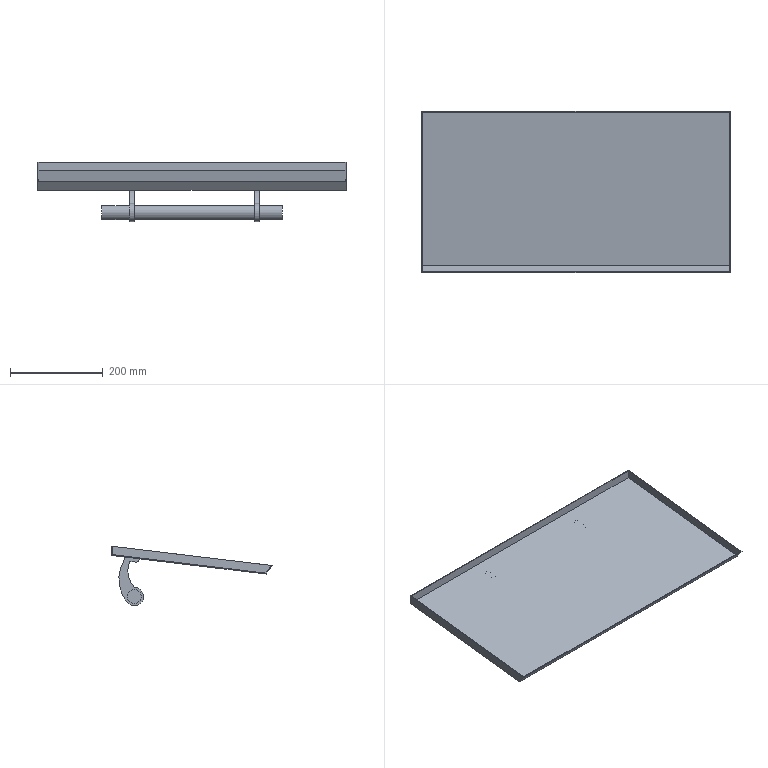Part | SolidWorks | features ICE 5, Extrusion 1, LPattern 1 | 1 solid | 35 faces | box 665 x 347.491 x 128.669 mm | volume 843762 mm3 | plane 21 | cylinder 10 | spline 4 | commonest cylinder face diameters 30 x6 14 x2 40 x2
STEP:
#1=CARTESIAN_POINT('',(-135.5,-49.466,-103.669));
#2=VERTEX_POINT('',#1);
#3=CARTESIAN_POINT('',(-135.5,-49.466,-73.669));
#4=VERTEX_POINT('',#3);
#5=CARTESIAN_POINT('',(-135.5,-49.466,-88.669));
#6=DIRECTION('',(1.,0.,0.));
#7=DIRECTION('',(0.,0.,-1.));
#8=AXIS2_PLACEMENT_3D('',#5,#6,#7);
#9=CIRCLE('',#8,15.);
#10=EDGE_CURVE('',#2,#4,#9,.T.);
#11=ORIENTED_EDGE('',*,*,#10,.F.);
#12=CARTESIAN_POINT('',(-185.5,-49.466,-103.669));
#13=VERTEX_POINT('',#12);
#14=CARTESIAN_POINT('',(-135.5,-49.466,-103.669));
#15=DIRECTION('',(-1.,0.,0.));
#16=VECTOR('',#15,1000.);
#17=LINE('',#14,#16);
#18=EDGE_CURVE('',#2,#13,#17,.T.);
#19=ORIENTED_EDGE('',*,*,#18,.T.);
#20=CARTESIAN_POINT('',(-185.5,-49.466,-73.669));
#21=VERTEX_POINT('',#20);
#22=CARTESIAN_POINT('',(-185.5,-49.466,-88.669));
#23=DIRECTION('',(1.,0.,0.));
#24=DIRECTION('',(0.,0.,-1.));
#25=AXIS2_PLACEMENT_3D('',#22,#23,#24);
#26=CIRCLE('',#25,15.);
#27=EDGE_CURVE('',#13,#21,#26,.T.);
#28=ORIENTED_EDGE('',*,*,#27,.T.);
#29=CARTESIAN_POINT('',(-135.5,-49.466,-73.669));
#30=DIRECTION('',(-1.,0.,0.));
#31=VECTOR('',#30,1000.);
#32=LINE('',#29,#31);
#33=EDGE_CURVE('',#4,#21,#32,.T.);
#34=ORIENTED_EDGE('',*,*,#33,.F.);
#35=EDGE_LOOP('',(#11,#19,#28,#34));
#36=FACE_OUTER_BOUND('',#35,.T.);
#37=CARTESIAN_POINT('',(-135.5,-49.466,-88.669));
#38=DIRECTION('',(-1.,0.,0.));
#39=DIRECTION('',(0.,0.,1.));
#40=AXIS2_PLACEMENT_3D('',#37,#38,#39);
#41=CYLINDRICAL_SURFACE('',#40,15.);
#42=ADVANCED_FACE('',(#36),#41,.T.);
#43=CARTESIAN_POINT('',(-455.5,-49.466,-103.669));
#44=VERTEX_POINT('',#43);
#45=CARTESIAN_POINT('',(-455.5,-49.466,-73.669));
#46=VERTEX_POINT('',#45);
#47=CARTESIAN_POINT('',(-455.5,-49.466,-88.669));
#48=DIRECTION('',(1.,0.,0.));
#49=DIRECTION('',(0.,0.,-1.));
#50=AXIS2_PLACEMENT_3D('',#47,#48,#49);
#51=CIRCLE('',#50,15.);
#52=EDGE_CURVE('',#44,#46,#51,.T.);
#53=ORIENTED_EDGE('',*,*,#52,.T.);
#54=CARTESIAN_POINT('',(-195.5,-49.466,-73.669));
#55=VERTEX_POINT('',#54);
#56=CARTESIAN_POINT('',(-525.5,-49.466,-73.669));
#57=DIRECTION('',(1.,0.,0.));
#58=VECTOR('',#57,1000.);
#59=LINE('',#56,#58);
#60=EDGE_CURVE('',#46,#55,#59,.T.);
#61=ORIENTED_EDGE('',*,*,#60,.T.);
#62=CARTESIAN_POINT('',(-195.5,-49.466,-103.669));
#63=VERTEX_POINT('',#62);
#64=CARTESIAN_POINT('',(-195.5,-49.466,-88.669));
#65=DIRECTION('',(1.,0.,0.));
#66=DIRECTION('',(0.,0.,-1.));
#67=AXIS2_PLACEMENT_3D('',#64,#65,#66);
#68=CIRCLE('',#67,15.);
#69=EDGE_CURVE('',#63,#55,#68,.T.);
#70=ORIENTED_EDGE('',*,*,#69,.F.);
#71=CARTESIAN_POINT('',(-525.5,-49.466,-103.669));
#72=DIRECTION('',(1.,0.,0.));
#73=VECTOR('',#72,1000.);
#74=LINE('',#71,#73);
#75=EDGE_CURVE('',#44,#63,#74,.T.);
#76=ORIENTED_EDGE('',*,*,#75,.F.);
#77=EDGE_LOOP('',(#53,#61,#70,#76));
#78=FACE_OUTER_BOUND('',#77,.T.);
#79=CARTESIAN_POINT('',(-525.5,-49.466,-88.669));
#80=DIRECTION('',(1.,0.,0.));
#81=DIRECTION('',(0.,0.,-1.));
#82=AXIS2_PLACEMENT_3D('',#79,#80,#81);
#83=CYLINDRICAL_SURFACE('',#82,15.);
#84=ADVANCED_FACE('',(#78),#83,.T.);
#85=CARTESIAN_POINT('',(-525.5,-49.466,-103.669));
#86=VERTEX_POINT('',#85);
#87=CARTESIAN_POINT('',(-525.5,-49.466,-73.669));
#88=VERTEX_POINT('',#87);
#89=CARTESIAN_POINT('',(-525.5,-49.466,-88.669));
#90=DIRECTION('',(1.,0.,0.));
#91=DIRECTION('',(0.,0.,-1.));
#92=AXIS2_PLACEMENT_3D('',#89,#90,#91);
#93=CIRCLE('',#92,15.);
#94=EDGE_CURVE('',#86,#88,#93,.T.);
#95=ORIENTED_EDGE('',*,*,#94,.T.);
#96=CARTESIAN_POINT('',(-465.5,-49.466,-73.669));
#97=VERTEX_POINT('',#96);
#98=CARTESIAN_POINT('',(-525.5,-49.466,-73.669));
#99=DIRECTION('',(1.,0.,0.));
#100=VECTOR('',#99,1000.);
#101=LINE('',#98,#100);
#102=EDGE_CURVE('',#88,#97,#101,.T.);
#103=ORIENTED_EDGE('',*,*,#102,.T.);
#104=CARTESIAN_POINT('',(-465.5,-49.466,-103.669));
#105=VERTEX_POINT('',#104);
#106=CARTESIAN_POINT('',(-465.5,-49.466,-88.669));
#107=DIRECTION('',(1.,0.,0.));
#108=DIRECTION('',(0.,0.,-1.));
#109=AXIS2_PLACEMENT_3D('',#106,#107,#108);
#110=CIRCLE('',#109,15.);
#111=EDGE_CURVE('',#105,#97,#110,.T.);
#112=ORIENTED_EDGE('',*,*,#111,.F.);
#113=CARTESIAN_POINT('',(-525.5,-49.466,-103.669));
#114=DIRECTION('',(1.,0.,0.));
#115=VECTOR('',#114,1000.);
#116=LINE('',#113,#115);
#117=EDGE_CURVE('',#86,#105,#116,.T.);
#118=ORIENTED_EDGE('',*,*,#117,.F.);
#119=EDGE_LOOP('',(#95,#103,#112,#118));
#120=FACE_OUTER_BOUND('',#119,.T.);
#121=CARTESIAN_POINT('',(-525.5,-49.466,-88.669));
#122=DIRECTION('',(1.,0.,0.));
#123=DIRECTION('',(0.,0.,-1.));
#124=AXIS2_PLACEMENT_3D('',#121,#122,#123);
#125=CYLINDRICAL_SURFACE('',#124,15.);
#126=ADVANCED_FACE('',(#120),#125,.T.);
#127=CARTESIAN_POINT('',(0.,-2.,1.774));
#128=VERTEX_POINT('',#127);
#129=CARTESIAN_POINT('',(0.,-2.,19.759));
#130=VERTEX_POINT('',#129);
#131=CARTESIAN_POINT('',(0.,-2.,1.774));
#132=DIRECTION('',(0.,0.,1.));
#133=VECTOR('',#132,1000.);
#134=LINE('',#131,#133);
#135=EDGE_CURVE('',#128,#130,#134,.T.);
#136=ORIENTED_EDGE('',*,*,#135,.F.);
#137=CARTESIAN_POINT('',(0.,-332.828,-38.054));
#138=VERTEX_POINT('',#137);
#139=CARTESIAN_POINT('',(0.,-332.828,-38.054));
#140=DIRECTION('',(0.,0.9928,0.1195));
#141=VECTOR('',#140,1000.);
#142=LINE('',#139,#141);
#143=EDGE_CURVE('',#138,#128,#142,.T.);
#144=ORIENTED_EDGE('',*,*,#143,.F.);
#145=CARTESIAN_POINT('',(0.,-345.198,-21.558));
#146=VERTEX_POINT('',#145);
#147=CARTESIAN_POINT('',(0.,-345.198,-21.558));
#148=DIRECTION('',(0.,0.5999,-0.8001));
#149=VECTOR('',#148,1000.);
#150=LINE('',#147,#149);
#151=EDGE_CURVE('',#146,#138,#150,.T.);
#152=ORIENTED_EDGE('',*,*,#151,.F.);
#153=CARTESIAN_POINT('',(0.,0.,20.));
#154=DIRECTION('',(0.,-0.9928,-0.1195));
#155=VECTOR('',#154,1000.);
#156=LINE('',#153,#155);
#157=EDGE_CURVE('',#130,#146,#156,.T.);
#158=ORIENTED_EDGE('',*,*,#157,.F.);
#159=EDGE_LOOP('',(#136,#144,#152,#158));
#160=FACE_OUTER_BOUND('',#159,.T.);
#161=CARTESIAN_POINT('',(0.,0.,0.));
#162=DIRECTION('',(1.,0.,0.));
#163=DIRECTION('',(0.,0.,-1.));
#164=AXIS2_PLACEMENT_3D('',#161,#162,#163);
#165=PLANE('',#164);
#166=ADVANCED_FACE('',(#160),#165,.F.);
#167=CARTESIAN_POINT('',(-455.5,-60.424,-7.274));
#168=VERTEX_POINT('',#167);
#169=CARTESIAN_POINT('',(-465.5,-60.424,-7.274));
#170=VERTEX_POINT('',#169);
#171=CARTESIAN_POINT('',(-455.5,-60.424,-7.274));
#172=DIRECTION('',(-1.,0.,0.));
#173=VECTOR('',#172,1000.);
#174=LINE('',#171,#173);
#175=EDGE_CURVE('',#168,#170,#174,.T.);
#176=ORIENTED_EDGE('',*,*,#175,.F.);
#177=CARTESIAN_POINT('',(-455.5,-29.965,-3.607));
#178=VERTEX_POINT('',#177);
#179=CARTESIAN_POINT('',(-455.5,0.,0.));
#180=DIRECTION('',(0.,0.9928,0.1195));
#181=VECTOR('',#180,1000.);
#182=LINE('',#179,#181);
#183=EDGE_CURVE('',#168,#178,#182,.T.);
#184=ORIENTED_EDGE('',*,*,#183,.T.);
#185=CARTESIAN_POINT('',(-465.5,-29.965,-3.607));
#186=VERTEX_POINT('',#185);
#187=CARTESIAN_POINT('',(-455.5,-29.965,-3.607));
#188=DIRECTION('',(-1.,0.,0.));
#189=VECTOR('',#188,1000.);
#190=LINE('',#187,#189);
#191=EDGE_CURVE('',#178,#186,#190,.T.);
#192=ORIENTED_EDGE('',*,*,#191,.T.);
#193=CARTESIAN_POINT('',(-465.5,0.,0.));
#194=DIRECTION('',(0.,0.9928,0.1195));
#195=VECTOR('',#194,1000.);
#196=LINE('',#193,#195);
#197=EDGE_CURVE('',#170,#186,#196,.T.);
#198=ORIENTED_EDGE('',*,*,#197,.F.);
#199=EDGE_LOOP('',(#176,#184,#192,#198));
#200=FACE_BOUND('',#199,.T.);
#201=CARTESIAN_POINT('',(-185.5,-60.424,-7.274));
#202=VERTEX_POINT('',#201);
#203=CARTESIAN_POINT('',(-195.5,-60.424,-7.274));
#204=VERTEX_POINT('',#203);
#205=CARTESIAN_POINT('',(-185.5,-60.424,-7.274));
#206=DIRECTION('',(-1.,0.,0.));
#207=VECTOR('',#206,1000.);
#208=LINE('',#205,#207);
#209=EDGE_CURVE('',#202,#204,#208,.T.);
#210=ORIENTED_EDGE('',*,*,#209,.F.);
#211=CARTESIAN_POINT('',(-185.5,-29.965,-3.607));
#212=VERTEX_POINT('',#211);
#213=CARTESIAN_POINT('',(-185.5,0.,0.));
#214=DIRECTION('',(0.,0.9928,0.1195));
#215=VECTOR('',#214,1000.);
#216=LINE('',#213,#215);
#217=EDGE_CURVE('',#202,#212,#216,.T.);
#218=ORIENTED_EDGE('',*,*,#217,.T.);
#219=CARTESIAN_POINT('',(-195.5,-29.965,-3.607));
#220=VERTEX_POINT('',#219);
#221=CARTESIAN_POINT('',(-185.5,-29.965,-3.607));
#222=DIRECTION('',(-1.,0.,0.));
#223=VECTOR('',#222,1000.);
#224=LINE('',#221,#223);
#225=EDGE_CURVE('',#212,#220,#224,.T.);
#226=ORIENTED_EDGE('',*,*,#225,.T.);
#227=CARTESIAN_POINT('',(-195.5,0.,0.));
#228=DIRECTION('',(0.,0.9928,0.1195));
#229=VECTOR('',#228,1000.);
#230=LINE('',#227,#229);
#231=EDGE_CURVE('',#204,#220,#230,.T.);
#232=ORIENTED_EDGE('',*,*,#231,.F.);
#233=EDGE_LOOP('',(#210,#218,#226,#232));
#234=FACE_BOUND('',#233,.T.);
#235=CARTESIAN_POINT('',(2.,-333.735,-40.178));
#236=VERTEX_POINT('',#235);
#237=CARTESIAN_POINT('',(-663.,-333.735,-40.178));
#238=VERTEX_POINT('',#237);
#239=CARTESIAN_POINT('',(2.,-333.735,-40.178));
#240=DIRECTION('',(-1.,0.,0.));
#241=VECTOR('',#240,1000.);
#242=LINE('',#239,#241);
#243=EDGE_CURVE('',#236,#238,#242,.T.);
#244=ORIENTED_EDGE('',*,*,#243,.T.);
#245=CARTESIAN_POINT('',(-663.,0.,0.));
#246=VERTEX_POINT('',#245);
#247=CARTESIAN_POINT('',(-663.,0.,0.));
#248=DIRECTION('',(0.,-0.9928,-0.1195));
#249=VECTOR('',#248,1000.);
#250=LINE('',#247,#249);
#251=EDGE_CURVE('',#246,#238,#250,.T.);
#252=ORIENTED_EDGE('',*,*,#251,.F.);
#253=CARTESIAN_POINT('',(2.,0.,0.));
#254=VERTEX_POINT('',#253);
#255=CARTESIAN_POINT('',(2.,0.,0.));
#256=DIRECTION('',(-1.,0.,0.));
#257=VECTOR('',#256,1000.);
#258=LINE('',#255,#257);
#259=EDGE_CURVE('',#254,#246,#258,.T.);
#260=ORIENTED_EDGE('',*,*,#259,.F.);
#261=CARTESIAN_POINT('',(2.,-333.735,-40.178));
#262=DIRECTION('',(0.,0.9928,0.1195));
#263=VECTOR('',#262,1000.);
#264=LINE('',#261,#263);
#265=EDGE_CURVE('',#236,#254,#264,.T.);
#266=ORIENTED_EDGE('',*,*,#265,.F.);
#267=EDGE_LOOP('',(#244,#252,#260,#266));
#268=FACE_OUTER_BOUND('',#267,.T.);
#269=CARTESIAN_POINT('',(2.,-333.735,-40.178));
#270=DIRECTION('',(0.,-0.1195,0.9928));
#271=DIRECTION('',(0.,-0.9928,-0.1195));
#272=AXIS2_PLACEMENT_3D('',#269,#270,#271);
#273=PLANE('',#272);
#274=ADVANCED_FACE('',(#200,#234,#268),#273,.F.);
#275=ORIENTED_EDGE('',*,*,#259,.T.);
#276=CARTESIAN_POINT('',(-663.,0.,20.));
#277=VERTEX_POINT('',#276);
#278=CARTESIAN_POINT('',(-663.,0.,20.));
#279=DIRECTION('',(0.,0.,-1.));
#280=VECTOR('',#279,1000.);
#281=LINE('',#278,#280);
#282=EDGE_CURVE('',#277,#246,#281,.T.);
#283=ORIENTED_EDGE('',*,*,#282,.F.);
#284=CARTESIAN_POINT('',(2.,0.,20.));
#285=VERTEX_POINT('',#284);
#286=CARTESIAN_POINT('',(2.,0.,20.));
#287=DIRECTION('',(-1.,0.,0.));
#288=VECTOR('',#287,1000.);
#289=LINE('',#286,#288);
#290=EDGE_CURVE('',#285,#277,#289,.T.);
#291=ORIENTED_EDGE('',*,*,#290,.F.);
#292=CARTESIAN_POINT('',(2.,0.,0.));
#293=DIRECTION('',(0.,0.,1.));
#294=VECTOR('',#293,1000.);
#295=LINE('',#292,#294);
#296=EDGE_CURVE('',#254,#285,#295,.T.);
#297=ORIENTED_EDGE('',*,*,#296,.F.);
#298=EDGE_LOOP('',(#275,#283,#291,#297));
#299=FACE_OUTER_BOUND('',#298,.T.);
#300=CARTESIAN_POINT('',(2.,0.,0.));
#301=DIRECTION('',(0.,-1.,0.));
#302=DIRECTION('',(0.,0.,-1.));
#303=AXIS2_PLACEMENT_3D('',#300,#301,#302);
#304=PLANE('',#303);
#305=ADVANCED_FACE('',(#299),#304,.F.);
#306=CARTESIAN_POINT('',(-661.,-345.198,-21.558));
#307=VERTEX_POINT('',#306);
#308=CARTESIAN_POINT('',(-661.,-345.198,-21.558));
#309=DIRECTION('',(1.,0.,0.));
#310=VECTOR('',#309,1000.);
#311=LINE('',#308,#310);
#312=EDGE_CURVE('',#307,#146,#311,.T.);
#313=ORIENTED_EDGE('',*,*,#312,.F.);
#314=CARTESIAN_POINT('',(-661.,-2.,19.759));
#315=VERTEX_POINT('',#314);
#316=CARTESIAN_POINT('',(-661.,-347.491,-21.834));
#317=DIRECTION('',(0.,0.9928,0.1195));
#318=VECTOR('',#317,1000.);
#319=LINE('',#316,#318);
#320=EDGE_CURVE('',#307,#315,#319,.T.);
#321=ORIENTED_EDGE('',*,*,#320,.T.);
#322=CARTESIAN_POINT('',(-661.,-2.,19.759));
#323=DIRECTION('',(1.,0.,0.));
#324=VECTOR('',#323,1000.);
#325=LINE('',#322,#324);
#326=EDGE_CURVE('',#315,#130,#325,.T.);
#327=ORIENTED_EDGE('',*,*,#326,.T.);
#328=ORIENTED_EDGE('',*,*,#157,.T.);
#329=EDGE_LOOP('',(#313,#321,#327,#328));
#330=FACE_BOUND('',#329,.T.);
#331=ORIENTED_EDGE('',*,*,#290,.T.);
#332=CARTESIAN_POINT('',(-663.,-347.491,-21.834));
#333=VERTEX_POINT('',#332);
#334=CARTESIAN_POINT('',(-663.,-347.491,-21.834));
#335=DIRECTION('',(0.,0.9928,0.1195));
#336=VECTOR('',#335,1000.);
#337=LINE('',#334,#336);
#338=EDGE_CURVE('',#333,#277,#337,.T.);
#339=ORIENTED_EDGE('',*,*,#338,.F.);
#340=CARTESIAN_POINT('',(2.,-347.491,-21.834));
#341=VERTEX_POINT('',#340);
#342=CARTESIAN_POINT('',(2.,-347.491,-21.834));
#343=DIRECTION('',(-1.,0.,0.));
#344=VECTOR('',#343,1000.);
#345=LINE('',#342,#344);
#346=EDGE_CURVE('',#341,#333,#345,.T.);
#347=ORIENTED_EDGE('',*,*,#346,.F.);
#348=CARTESIAN_POINT('',(2.,0.,20.));
#349=DIRECTION('',(0.,-0.9928,-0.1195));
#350=VECTOR('',#349,1000.);
#351=LINE('',#348,#350);
#352=EDGE_CURVE('',#285,#341,#351,.T.);
#353=ORIENTED_EDGE('',*,*,#352,.F.);
#354=EDGE_LOOP('',(#331,#339,#347,#353));
#355=FACE_OUTER_BOUND('',#354,.T.);
#356=CARTESIAN_POINT('',(2.,0.,20.));
#357=DIRECTION('',(0.,0.1195,-0.9928));
#358=DIRECTION('',(0.,0.9928,0.1195));
#359=AXIS2_PLACEMENT_3D('',#356,#357,#358);
#360=PLANE('',#359);
#361=ADVANCED_FACE('',(#330,#355),#360,.F.);
#362=ORIENTED_EDGE('',*,*,#346,.T.);
#363=CARTESIAN_POINT('',(-663.,-333.735,-40.178));
#364=DIRECTION('',(0.,-0.5999,0.8001));
#365=VECTOR('',#364,1000.);
#366=LINE('',#363,#365);
#367=EDGE_CURVE('',#238,#333,#366,.T.);
#368=ORIENTED_EDGE('',*,*,#367,.F.);
#369=ORIENTED_EDGE('',*,*,#243,.F.);
#370=CARTESIAN_POINT('',(2.,-347.491,-21.834));
#371=DIRECTION('',(0.,0.5999,-0.8001));
#372=VECTOR('',#371,1000.);
#373=LINE('',#370,#372);
#374=EDGE_CURVE('',#341,#236,#373,.T.);
#375=ORIENTED_EDGE('',*,*,#374,.F.);
#376=EDGE_LOOP('',(#362,#368,#369,#375));
#377=FACE_OUTER_BOUND('',#376,.T.);
#378=CARTESIAN_POINT('',(2.,-347.491,-21.834));
#379=DIRECTION('',(0.,0.8001,0.5999));
#380=DIRECTION('',(0.,-0.5999,0.8001));
#381=AXIS2_PLACEMENT_3D('',#378,#379,#380);
#382=PLANE('',#381);
#383=ADVANCED_FACE('',(#377),#382,.F.);
#384=ORIENTED_EDGE('',*,*,#265,.T.);
#385=ORIENTED_EDGE('',*,*,#296,.T.);
#386=ORIENTED_EDGE('',*,*,#352,.T.);
#387=ORIENTED_EDGE('',*,*,#374,.T.);
#388=EDGE_LOOP('',(#384,#385,#386,#387));
#389=FACE_OUTER_BOUND('',#388,.T.);
#390=CARTESIAN_POINT('',(2.,0.,0.));
#391=DIRECTION('',(1.,0.,0.));
#392=DIRECTION('',(0.,0.,-1.));
#393=AXIS2_PLACEMENT_3D('',#390,#391,#392);
#394=PLANE('',#393);
#395=ADVANCED_FACE('',(#389),#394,.T.);
#396=ORIENTED_EDGE('',*,*,#151,.T.);
#397=CARTESIAN_POINT('',(-661.,-332.828,-38.054));
#398=VERTEX_POINT('',#397);
#399=CARTESIAN_POINT('',(-661.,-332.828,-38.054));
#400=DIRECTION('',(1.,0.,0.));
#401=VECTOR('',#400,1000.);
#402=LINE('',#399,#401);
#403=EDGE_CURVE('',#398,#138,#402,.T.);
#404=ORIENTED_EDGE('',*,*,#403,.F.);
#405=CARTESIAN_POINT('',(-661.,-345.198,-21.558));
#406=DIRECTION('',(0.,0.5999,-0.8001));
#407=VECTOR('',#406,1000.);
#408=LINE('',#405,#407);
#409=EDGE_CURVE('',#307,#398,#408,.T.);
#410=ORIENTED_EDGE('',*,*,#409,.F.);
#411=ORIENTED_EDGE('',*,*,#312,.T.);
#412=EDGE_LOOP('',(#396,#404,#410,#411));
#413=FACE_OUTER_BOUND('',#412,.T.);
#414=CARTESIAN_POINT('',(-661.,-345.198,-21.558));
#415=DIRECTION('',(0.,-0.8001,-0.5999));
#416=DIRECTION('',(0.,0.5999,-0.8001));
#417=AXIS2_PLACEMENT_3D('',#414,#415,#416);
#418=PLANE('',#417);
#419=ADVANCED_FACE('',(#413),#418,.F.);
#420=ORIENTED_EDGE('',*,*,#143,.T.);
#421=CARTESIAN_POINT('',(-661.,-2.,1.774));
#422=VERTEX_POINT('',#421);
#423=CARTESIAN_POINT('',(-661.,-2.,1.774));
#424=DIRECTION('',(1.,0.,0.));
#425=VECTOR('',#424,1000.);
#426=LINE('',#423,#425);
#427=EDGE_CURVE('',#422,#128,#426,.T.);
#428=ORIENTED_EDGE('',*,*,#427,.F.);
#429=CARTESIAN_POINT('',(-661.,-332.828,-38.054));
#430=DIRECTION('',(0.,0.9928,0.1195));
#431=VECTOR('',#430,1000.);
#432=LINE('',#429,#431);
#433=EDGE_CURVE('',#398,#422,#432,.T.);
#434=ORIENTED_EDGE('',*,*,#433,.F.);
#435=ORIENTED_EDGE('',*,*,#403,.T.);
#436=EDGE_LOOP('',(#420,#428,#434,#435));
#437=FACE_OUTER_BOUND('',#436,.T.);
#438=CARTESIAN_POINT('',(-661.,-332.828,-38.054));
#439=DIRECTION('',(0.,0.1195,-0.9928));
#440=DIRECTION('',(0.,0.9928,0.1195));
#441=AXIS2_PLACEMENT_3D('',#438,#439,#440);
#442=PLANE('',#441);
#443=ADVANCED_FACE('',(#437),#442,.F.);
#444=ORIENTED_EDGE('',*,*,#135,.T.);
#445=ORIENTED_EDGE('',*,*,#326,.F.);
#446=CARTESIAN_POINT('',(-661.,-2.,1.774));
#447=DIRECTION('',(0.,0.,1.));
#448=VECTOR('',#447,1000.);
#449=LINE('',#446,#448);
#450=EDGE_CURVE('',#422,#315,#449,.T.);
#451=ORIENTED_EDGE('',*,*,#450,.F.);
#452=ORIENTED_EDGE('',*,*,#427,.T.);
#453=EDGE_LOOP('',(#444,#445,#451,#452));
#454=FACE_OUTER_BOUND('',#453,.T.);
#455=CARTESIAN_POINT('',(-661.,-2.,1.774));
#456=DIRECTION('',(0.,1.,0.));
#457=DIRECTION('',(0.,0.,1.));
#458=AXIS2_PLACEMENT_3D('',#455,#456,#457);
#459=PLANE('',#458);
#460=ADVANCED_FACE('',(#454),#459,.F.);
#461=ORIENTED_EDGE('',*,*,#251,.T.);
#462=ORIENTED_EDGE('',*,*,#367,.T.);
#463=ORIENTED_EDGE('',*,*,#338,.T.);
#464=ORIENTED_EDGE('',*,*,#282,.T.);
#465=EDGE_LOOP('',(#461,#462,#463,#464));
#466=FACE_OUTER_BOUND('',#465,.T.);
#467=CARTESIAN_POINT('',(-663.,0.,0.));
#468=DIRECTION('',(1.,0.,0.));
#469=DIRECTION('',(0.,0.,-1.));
#470=AXIS2_PLACEMENT_3D('',#467,#468,#469);
#471=PLANE('',#470);
#472=ADVANCED_FACE('',(#466),#471,.F.);
#473=ORIENTED_EDGE('',*,*,#320,.F.);
#474=ORIENTED_EDGE('',*,*,#409,.T.);
#475=ORIENTED_EDGE('',*,*,#433,.T.);
#476=ORIENTED_EDGE('',*,*,#450,.T.);
#477=EDGE_LOOP('',(#473,#474,#475,#476));
#478=FACE_OUTER_BOUND('',#477,.T.);
#479=CARTESIAN_POINT('',(-661.,0.,0.));
#480=DIRECTION('',(1.,0.,0.));
#481=DIRECTION('',(0.,0.,-1.));
#482=AXIS2_PLACEMENT_3D('',#479,#480,#481);
#483=PLANE('',#482);
#484=ADVANCED_FACE('',(#478),#483,.T.);
#485=CARTESIAN_POINT('',(-195.5,-49.466,-68.669));
#486=VERTEX_POINT('',#485);
#487=CARTESIAN_POINT('',(-195.5,-33.713,-100.991));
#488=VERTEX_POINT('',#487);
#489=CARTESIAN_POINT('',(-195.5,-49.466,-88.669));
#490=DIRECTION('',(1.,0.,0.));
#491=DIRECTION('',(0.,0.,-1.));
#492=AXIS2_PLACEMENT_3D('',#489,#490,#491);
#493=CIRCLE('',#492,20.);
#494=EDGE_CURVE('',#486,#488,#493,.T.);
#495=ORIENTED_EDGE('',*,*,#494,.T.);
#496=CARTESIAN_POINT('',(-185.5,-33.713,-100.991));
#497=VERTEX_POINT('',#496);
#498=CARTESIAN_POINT('',(-185.5,-33.713,-100.991));
#499=DIRECTION('',(-1.,0.,0.));
#500=VECTOR('',#499,1000.);
#501=LINE('',#498,#500);
#502=EDGE_CURVE('',#497,#488,#501,.T.);
#503=ORIENTED_EDGE('',*,*,#502,.F.);
#504=CARTESIAN_POINT('',(-185.5,-49.466,-68.669));
#505=VERTEX_POINT('',#504);
#506=CARTESIAN_POINT('',(-185.5,-49.466,-88.669));
#507=DIRECTION('',(1.,0.,0.));
#508=DIRECTION('',(0.,0.,-1.));
#509=AXIS2_PLACEMENT_3D('',#506,#507,#508);
#510=CIRCLE('',#509,20.);
#511=EDGE_CURVE('',#505,#497,#510,.T.);
#512=ORIENTED_EDGE('',*,*,#511,.F.);
#513=CARTESIAN_POINT('',(-185.5,-49.466,-68.669));
#514=DIRECTION('',(-1.,0.,0.));
#515=VECTOR('',#514,1000.);
#516=LINE('',#513,#515);
#517=EDGE_CURVE('',#505,#486,#516,.T.);
#518=ORIENTED_EDGE('',*,*,#517,.T.);
#519=EDGE_LOOP('',(#495,#503,#512,#518));
#520=FACE_OUTER_BOUND('',#519,.T.);
#521=CARTESIAN_POINT('',(-185.5,-49.466,-88.669));
#522=DIRECTION('',(-1.,0.,0.));
#523=DIRECTION('',(0.,0.,1.));
#524=AXIS2_PLACEMENT_3D('',#521,#522,#523);
#525=CYLINDRICAL_SURFACE('',#524,20.);
#526=ADVANCED_FACE('',(#520),#525,.T.);
#527=CARTESIAN_POINT('',(-195.5,-29.965,-3.607));
#528=CARTESIAN_POINT('',(-195.5,-12.413,-33.423));
#529=CARTESIAN_POINT('',(-195.5,-8.887,-69.251));
#530=CARTESIAN_POINT('',(-195.5,-33.713,-100.991));
#531=B_SPLINE_CURVE_WITH_KNOTS('',3,(#527,#528,#529,#530),.UNSPECIFIED.,.F.,.F.,(4,4),(0.,1.),.UNSPECIFIED.);
#532=EDGE_CURVE('',#220,#488,#531,.T.);
#533=ORIENTED_EDGE('',*,*,#532,.F.);
#534=ORIENTED_EDGE('',*,*,#225,.F.);
#535=CARTESIAN_POINT('',(-185.5,-29.965,-3.607));
#536=CARTESIAN_POINT('',(-185.5,-12.413,-33.423));
#537=CARTESIAN_POINT('',(-185.5,-8.887,-69.251));
#538=CARTESIAN_POINT('',(-185.5,-33.713,-100.991));
#539=B_SPLINE_CURVE_WITH_KNOTS('',3,(#535,#536,#537,#538),.UNSPECIFIED.,.F.,.F.,(4,4),(0.,1.),.UNSPECIFIED.);
#540=EDGE_CURVE('',#212,#497,#539,.T.);
#541=ORIENTED_EDGE('',*,*,#540,.T.);
#542=ORIENTED_EDGE('',*,*,#502,.T.);
#543=EDGE_LOOP('',(#533,#534,#541,#542));
#544=FACE_OUTER_BOUND('',#543,.T.);
#545=CARTESIAN_POINT('',(-185.5,-29.965,-3.607));
#546=CARTESIAN_POINT('',(-195.5,-29.965,-3.607));
#547=CARTESIAN_POINT('',(-185.5,-12.413,-33.423));
#548=CARTESIAN_POINT('',(-195.5,-12.413,-33.423));
#549=CARTESIAN_POINT('',(-185.5,-8.887,-69.251));
#550=CARTESIAN_POINT('',(-195.5,-8.887,-69.251));
#551=CARTESIAN_POINT('',(-185.5,-33.713,-100.991));
#552=CARTESIAN_POINT('',(-195.5,-33.713,-100.991));
#553=B_SPLINE_SURFACE_WITH_KNOTS('',3,1,((#545,#546),(#547,#548),(#549,#550),(#551,#552)),.UNSPECIFIED.,.F.,.F.,.F.,(4,4),(2,2),(0.,1.),(0.,1.),.UNSPECIFIED.);
#554=ADVANCED_FACE('',(#544),#553,.T.);
#555=CARTESIAN_POINT('',(-195.5,-60.305,-8.267));
#556=VERTEX_POINT('',#555);
#557=CARTESIAN_POINT('',(-195.5,-60.424,-7.274));
#558=DIRECTION('',(0.,0.1195,-0.9928));
#559=VECTOR('',#558,1000.);
#560=LINE('',#557,#559);
#561=EDGE_CURVE('',#204,#556,#560,.T.);
#562=ORIENTED_EDGE('',*,*,#561,.T.);
#563=CARTESIAN_POINT('',(-185.5,-60.305,-8.267));
#564=VERTEX_POINT('',#563);
#565=CARTESIAN_POINT('',(-185.5,-60.305,-8.267));
#566=DIRECTION('',(-1.,0.,0.));
#567=VECTOR('',#566,1000.);
#568=LINE('',#565,#567);
#569=EDGE_CURVE('',#564,#556,#568,.T.);
#570=ORIENTED_EDGE('',*,*,#569,.F.);
#571=CARTESIAN_POINT('',(-185.5,-60.424,-7.274));
#572=DIRECTION('',(0.,0.1195,-0.9928));
#573=VECTOR('',#572,1000.);
#574=LINE('',#571,#573);
#575=EDGE_CURVE('',#202,#564,#574,.T.);
#576=ORIENTED_EDGE('',*,*,#575,.F.);
#577=ORIENTED_EDGE('',*,*,#209,.T.);
#578=EDGE_LOOP('',(#562,#570,#576,#577));
#579=FACE_OUTER_BOUND('',#578,.T.);
#580=CARTESIAN_POINT('',(-185.5,-60.424,-7.274));
#581=DIRECTION('',(0.,0.9928,0.1195));
#582=DIRECTION('',(0.,-0.1195,0.9928));
#583=AXIS2_PLACEMENT_3D('',#580,#581,#582);
#584=PLANE('',#583);
#585=ADVANCED_FACE('',(#579),#584,.F.);
#586=CARTESIAN_POINT('',(-195.5,-52.518,-14.38));
#587=VERTEX_POINT('',#586);
#588=CARTESIAN_POINT('',(-195.5,-53.355,-7.431));
#589=DIRECTION('',(-1.,0.,0.));
#590=DIRECTION('',(0.,0.,-1.));
#591=AXIS2_PLACEMENT_3D('',#588,#589,#590);
#592=CIRCLE('',#591,7.);
#593=EDGE_CURVE('',#587,#556,#592,.T.);
#594=ORIENTED_EDGE('',*,*,#593,.F.);
#595=CARTESIAN_POINT('',(-185.5,-52.518,-14.38));
#596=VERTEX_POINT('',#595);
#597=CARTESIAN_POINT('',(-185.5,-52.518,-14.38));
#598=DIRECTION('',(-1.,0.,0.));
#599=VECTOR('',#598,1000.);
#600=LINE('',#597,#599);
#601=EDGE_CURVE('',#596,#587,#600,.T.);
#602=ORIENTED_EDGE('',*,*,#601,.F.);
#603=CARTESIAN_POINT('',(-185.5,-53.355,-7.431));
#604=DIRECTION('',(-1.,0.,0.));
#605=DIRECTION('',(0.,0.,-1.));
#606=AXIS2_PLACEMENT_3D('',#603,#604,#605);
#607=CIRCLE('',#606,7.);
#608=EDGE_CURVE('',#596,#564,#607,.T.);
#609=ORIENTED_EDGE('',*,*,#608,.T.);
#610=ORIENTED_EDGE('',*,*,#569,.T.);
#611=EDGE_LOOP('',(#594,#602,#609,#610));
#612=FACE_OUTER_BOUND('',#611,.T.);
#613=CARTESIAN_POINT('',(-185.5,-53.355,-7.431));
#614=DIRECTION('',(-1.,0.,0.));
#615=DIRECTION('',(0.,0.,1.));
#616=AXIS2_PLACEMENT_3D('',#613,#614,#615);
#617=CYLINDRICAL_SURFACE('',#616,7.);
#618=ADVANCED_FACE('',(#612),#617,.T.);
#619=CARTESIAN_POINT('',(-195.5,-39.608,-12.826));
#620=VERTEX_POINT('',#619);
#621=CARTESIAN_POINT('',(-195.5,0.9562,-7.943));
#622=DIRECTION('',(0.,0.9928,0.1195));
#623=VECTOR('',#622,1000.);
#624=LINE('',#621,#623);
#625=EDGE_CURVE('',#587,#620,#624,.T.);
#626=ORIENTED_EDGE('',*,*,#625,.T.);
#627=CARTESIAN_POINT('',(-185.5,-39.608,-12.826));
#628=VERTEX_POINT('',#627);
#629=CARTESIAN_POINT('',(-185.5,-39.608,-12.826));
#630=DIRECTION('',(-1.,0.,0.));
#631=VECTOR('',#630,1000.);
#632=LINE('',#629,#631);
#633=EDGE_CURVE('',#628,#620,#632,.T.);
#634=ORIENTED_EDGE('',*,*,#633,.F.);
#635=CARTESIAN_POINT('',(-185.5,0.9562,-7.943));
#636=DIRECTION('',(0.,0.9928,0.1195));
#637=VECTOR('',#636,1000.);
#638=LINE('',#635,#637);
#639=EDGE_CURVE('',#596,#628,#638,.T.);
#640=ORIENTED_EDGE('',*,*,#639,.F.);
#641=ORIENTED_EDGE('',*,*,#601,.T.);
#642=EDGE_LOOP('',(#626,#634,#640,#641));
#643=FACE_OUTER_BOUND('',#642,.T.);
#644=CARTESIAN_POINT('',(-185.5,0.9562,-7.943));
#645=DIRECTION('',(0.,-0.1195,0.9928));
#646=DIRECTION('',(0.,-0.9928,-0.1195));
#647=AXIS2_PLACEMENT_3D('',#644,#645,#646);
#648=PLANE('',#647);
#649=ADVANCED_FACE('',(#643),#648,.F.);
#650=CARTESIAN_POINT('',(-195.5,-39.608,-12.826));
#651=CARTESIAN_POINT('',(-195.5,-27.323,-40.794));
#652=CARTESIAN_POINT('',(-195.5,-49.466,-68.669));
#653=B_SPLINE_CURVE_WITH_KNOTS('',2,(#650,#651,#652),.UNSPECIFIED.,.F.,.F.,(3,3),(0.,1.),.UNSPECIFIED.);
#654=EDGE_CURVE('',#620,#486,#653,.T.);
#655=ORIENTED_EDGE('',*,*,#654,.T.);
#656=ORIENTED_EDGE('',*,*,#517,.F.);
#657=CARTESIAN_POINT('',(-185.5,-39.608,-12.826));
#658=CARTESIAN_POINT('',(-185.5,-27.323,-40.794));
#659=CARTESIAN_POINT('',(-185.5,-49.466,-68.669));
#660=B_SPLINE_CURVE_WITH_KNOTS('',2,(#657,#658,#659),.UNSPECIFIED.,.F.,.F.,(3,3),(0.,1.),.UNSPECIFIED.);
#661=EDGE_CURVE('',#628,#505,#660,.T.);
#662=ORIENTED_EDGE('',*,*,#661,.F.);
#663=ORIENTED_EDGE('',*,*,#633,.T.);
#664=EDGE_LOOP('',(#655,#656,#662,#663));
#665=FACE_OUTER_BOUND('',#664,.T.);
#666=CARTESIAN_POINT('',(-185.5,-39.608,-12.826));
#667=CARTESIAN_POINT('',(-195.5,-39.608,-12.826));
#668=CARTESIAN_POINT('',(-185.5,-27.323,-40.794));
#669=CARTESIAN_POINT('',(-195.5,-27.323,-40.794));
#670=CARTESIAN_POINT('',(-185.5,-49.466,-68.669));
#671=CARTESIAN_POINT('',(-195.5,-49.466,-68.669));
#672=B_SPLINE_SURFACE_WITH_KNOTS('',2,1,((#666,#667),(#668,#669),(#670,#671)),.UNSPECIFIED.,.F.,.F.,.F.,(3,3),(2,2),(0.,1.),(0.,1.),.UNSPECIFIED.);
#673=ADVANCED_FACE('',(#665),#672,.F.);
#674=CARTESIAN_POINT('',(-185.5,-49.466,-88.669));
#675=DIRECTION('',(1.,0.,0.));
#676=DIRECTION('',(0.,0.,-1.));
#677=AXIS2_PLACEMENT_3D('',#674,#675,#676);
#678=CIRCLE('',#677,15.);
#679=EDGE_CURVE('',#21,#13,#678,.T.);
#680=ORIENTED_EDGE('',*,*,#679,.F.);
#681=ORIENTED_EDGE('',*,*,#27,.F.);
#682=EDGE_LOOP('',(#680,#681));
#683=FACE_BOUND('',#682,.T.);
#684=ORIENTED_EDGE('',*,*,#511,.T.);
#685=ORIENTED_EDGE('',*,*,#540,.F.);
#686=ORIENTED_EDGE('',*,*,#217,.F.);
#687=ORIENTED_EDGE('',*,*,#575,.T.);
#688=ORIENTED_EDGE('',*,*,#608,.F.);
#689=ORIENTED_EDGE('',*,*,#639,.T.);
#690=ORIENTED_EDGE('',*,*,#661,.T.);
#691=EDGE_LOOP('',(#684,#685,#686,#687,#688,#689,#690));
#692=FACE_OUTER_BOUND('',#691,.T.);
#693=CARTESIAN_POINT('',(-185.5,0.,0.));
#694=DIRECTION('',(1.,0.,0.));
#695=DIRECTION('',(0.,0.,-1.));
#696=AXIS2_PLACEMENT_3D('',#693,#694,#695);
#697=PLANE('',#696);
#698=ADVANCED_FACE('',(#683,#692),#697,.T.);
#699=ORIENTED_EDGE('',*,*,#69,.T.);
#700=CARTESIAN_POINT('',(-195.5,-49.466,-88.669));
#701=DIRECTION('',(1.,0.,0.));
#702=DIRECTION('',(0.,0.,-1.));
#703=AXIS2_PLACEMENT_3D('',#700,#701,#702);
#704=CIRCLE('',#703,15.);
#705=EDGE_CURVE('',#55,#63,#704,.T.);
#706=ORIENTED_EDGE('',*,*,#705,.T.);
#707=EDGE_LOOP('',(#699,#706));
#708=FACE_BOUND('',#707,.T.);
#709=ORIENTED_EDGE('',*,*,#494,.F.);
#710=ORIENTED_EDGE('',*,*,#654,.F.);
#711=ORIENTED_EDGE('',*,*,#625,.F.);
#712=ORIENTED_EDGE('',*,*,#593,.T.);
#713=ORIENTED_EDGE('',*,*,#561,.F.);
#714=ORIENTED_EDGE('',*,*,#231,.T.);
#715=ORIENTED_EDGE('',*,*,#532,.T.);
#716=EDGE_LOOP('',(#709,#710,#711,#712,#713,#714,#715));
#717=FACE_OUTER_BOUND('',#716,.T.);
#718=CARTESIAN_POINT('',(-195.5,0.,0.));
#719=DIRECTION('',(1.,0.,0.));
#720=DIRECTION('',(0.,0.,-1.));
#721=AXIS2_PLACEMENT_3D('',#718,#719,#720);
#722=PLANE('',#721);
#723=ADVANCED_FACE('',(#708,#717),#722,.F.);
#724=CARTESIAN_POINT('',(-465.5,-49.466,-68.669));
#725=VERTEX_POINT('',#724);
#726=CARTESIAN_POINT('',(-465.5,-33.713,-100.991));
#727=VERTEX_POINT('',#726);
#728=CARTESIAN_POINT('',(-465.5,-49.466,-88.669));
#729=DIRECTION('',(1.,0.,0.));
#730=DIRECTION('',(0.,0.,-1.));
#731=AXIS2_PLACEMENT_3D('',#728,#729,#730);
#732=CIRCLE('',#731,20.);
#733=EDGE_CURVE('',#725,#727,#732,.T.);
#734=ORIENTED_EDGE('',*,*,#733,.T.);
#735=CARTESIAN_POINT('',(-455.5,-33.713,-100.991));
#736=VERTEX_POINT('',#735);
#737=CARTESIAN_POINT('',(-455.5,-33.713,-100.991));
#738=DIRECTION('',(-1.,0.,0.));
#739=VECTOR('',#738,1000.);
#740=LINE('',#737,#739);
#741=EDGE_CURVE('',#736,#727,#740,.T.);
#742=ORIENTED_EDGE('',*,*,#741,.F.);
#743=CARTESIAN_POINT('',(-455.5,-49.466,-68.669));
#744=VERTEX_POINT('',#743);
#745=CARTESIAN_POINT('',(-455.5,-49.466,-88.669));
#746=DIRECTION('',(1.,0.,0.));
#747=DIRECTION('',(0.,0.,-1.));
#748=AXIS2_PLACEMENT_3D('',#745,#746,#747);
#749=CIRCLE('',#748,20.);
#750=EDGE_CURVE('',#744,#736,#749,.T.);
#751=ORIENTED_EDGE('',*,*,#750,.F.);
#752=CARTESIAN_POINT('',(-455.5,-49.466,-68.669));
#753=DIRECTION('',(-1.,0.,0.));
#754=VECTOR('',#753,1000.);
#755=LINE('',#752,#754);
#756=EDGE_CURVE('',#744,#725,#755,.T.);
#757=ORIENTED_EDGE('',*,*,#756,.T.);
#758=EDGE_LOOP('',(#734,#742,#751,#757));
#759=FACE_OUTER_BOUND('',#758,.T.);
#760=CARTESIAN_POINT('',(-455.5,-49.466,-88.669));
#761=DIRECTION('',(-1.,0.,0.));
#762=DIRECTION('',(0.,0.,1.));
#763=AXIS2_PLACEMENT_3D('',#760,#761,#762);
#764=CYLINDRICAL_SURFACE('',#763,20.);
#765=ADVANCED_FACE('',(#759),#764,.T.);
#766=CARTESIAN_POINT('',(-465.5,-29.965,-3.607));
#767=CARTESIAN_POINT('',(-465.5,-12.413,-33.423));
#768=CARTESIAN_POINT('',(-465.5,-8.887,-69.251));
#769=CARTESIAN_POINT('',(-465.5,-33.713,-100.991));
#770=B_SPLINE_CURVE_WITH_KNOTS('',3,(#766,#767,#768,#769),.UNSPECIFIED.,.F.,.F.,(4,4),(0.,1.),.UNSPECIFIED.);
#771=EDGE_CURVE('',#186,#727,#770,.T.);
#772=ORIENTED_EDGE('',*,*,#771,.F.);
#773=ORIENTED_EDGE('',*,*,#191,.F.);
#774=CARTESIAN_POINT('',(-455.5,-29.965,-3.607));
#775=CARTESIAN_POINT('',(-455.5,-12.413,-33.423));
#776=CARTESIAN_POINT('',(-455.5,-8.887,-69.251));
#777=CARTESIAN_POINT('',(-455.5,-33.713,-100.991));
#778=B_SPLINE_CURVE_WITH_KNOTS('',3,(#774,#775,#776,#777),.UNSPECIFIED.,.F.,.F.,(4,4),(0.,1.),.UNSPECIFIED.);
#779=EDGE_CURVE('',#178,#736,#778,.T.);
#780=ORIENTED_EDGE('',*,*,#779,.T.);
#781=ORIENTED_EDGE('',*,*,#741,.T.);
#782=EDGE_LOOP('',(#772,#773,#780,#781));
#783=FACE_OUTER_BOUND('',#782,.T.);
#784=CARTESIAN_POINT('',(-455.5,-29.965,-3.607));
#785=CARTESIAN_POINT('',(-465.5,-29.965,-3.607));
#786=CARTESIAN_POINT('',(-455.5,-12.413,-33.423));
#787=CARTESIAN_POINT('',(-465.5,-12.413,-33.423));
#788=CARTESIAN_POINT('',(-455.5,-8.887,-69.251));
#789=CARTESIAN_POINT('',(-465.5,-8.887,-69.251));
#790=CARTESIAN_POINT('',(-455.5,-33.713,-100.991));
#791=CARTESIAN_POINT('',(-465.5,-33.713,-100.991));
#792=B_SPLINE_SURFACE_WITH_KNOTS('',3,1,((#784,#785),(#786,#787),(#788,#789),(#790,#791)),.UNSPECIFIED.,.F.,.F.,.F.,(4,4),(2,2),(0.,1.),(0.,1.),.UNSPECIFIED.);
#793=ADVANCED_FACE('',(#783),#792,.T.);
#794=CARTESIAN_POINT('',(-465.5,-60.305,-8.267));
#795=VERTEX_POINT('',#794);
#796=CARTESIAN_POINT('',(-465.5,-60.424,-7.274));
#797=DIRECTION('',(0.,0.1195,-0.9928));
#798=VECTOR('',#797,1000.);
#799=LINE('',#796,#798);
#800=EDGE_CURVE('',#170,#795,#799,.T.);
#801=ORIENTED_EDGE('',*,*,#800,.T.);
#802=CARTESIAN_POINT('',(-455.5,-60.305,-8.267));
#803=VERTEX_POINT('',#802);
#804=CARTESIAN_POINT('',(-455.5,-60.305,-8.267));
#805=DIRECTION('',(-1.,0.,0.));
#806=VECTOR('',#805,1000.);
#807=LINE('',#804,#806);
#808=EDGE_CURVE('',#803,#795,#807,.T.);
#809=ORIENTED_EDGE('',*,*,#808,.F.);
#810=CARTESIAN_POINT('',(-455.5,-60.424,-7.274));
#811=DIRECTION('',(0.,0.1195,-0.9928));
#812=VECTOR('',#811,1000.);
#813=LINE('',#810,#812);
#814=EDGE_CURVE('',#168,#803,#813,.T.);
#815=ORIENTED_EDGE('',*,*,#814,.F.);
#816=ORIENTED_EDGE('',*,*,#175,.T.);
#817=EDGE_LOOP('',(#801,#809,#815,#816));
#818=FACE_OUTER_BOUND('',#817,.T.);
#819=CARTESIAN_POINT('',(-455.5,-60.424,-7.274));
#820=DIRECTION('',(0.,0.9928,0.1195));
#821=DIRECTION('',(0.,-0.1195,0.9928));
#822=AXIS2_PLACEMENT_3D('',#819,#820,#821);
#823=PLANE('',#822);
#824=ADVANCED_FACE('',(#818),#823,.F.);
#825=CARTESIAN_POINT('',(-465.5,-52.518,-14.38));
#826=VERTEX_POINT('',#825);
#827=CARTESIAN_POINT('',(-465.5,-53.355,-7.431));
#828=DIRECTION('',(-1.,0.,0.));
#829=DIRECTION('',(0.,0.,-1.));
#830=AXIS2_PLACEMENT_3D('',#827,#828,#829);
#831=CIRCLE('',#830,7.);
#832=EDGE_CURVE('',#826,#795,#831,.T.);
#833=ORIENTED_EDGE('',*,*,#832,.F.);
#834=CARTESIAN_POINT('',(-455.5,-52.518,-14.38));
#835=VERTEX_POINT('',#834);
#836=CARTESIAN_POINT('',(-455.5,-52.518,-14.38));
#837=DIRECTION('',(-1.,0.,0.));
#838=VECTOR('',#837,1000.);
#839=LINE('',#836,#838);
#840=EDGE_CURVE('',#835,#826,#839,.T.);
#841=ORIENTED_EDGE('',*,*,#840,.F.);
#842=CARTESIAN_POINT('',(-455.5,-53.355,-7.431));
#843=DIRECTION('',(-1.,0.,0.));
#844=DIRECTION('',(0.,0.,-1.));
#845=AXIS2_PLACEMENT_3D('',#842,#843,#844);
#846=CIRCLE('',#845,7.);
#847=EDGE_CURVE('',#835,#803,#846,.T.);
#848=ORIENTED_EDGE('',*,*,#847,.T.);
#849=ORIENTED_EDGE('',*,*,#808,.T.);
#850=EDGE_LOOP('',(#833,#841,#848,#849));
#851=FACE_OUTER_BOUND('',#850,.T.);
#852=CARTESIAN_POINT('',(-455.5,-53.355,-7.431));
#853=DIRECTION('',(-1.,0.,0.));
#854=DIRECTION('',(0.,0.,1.));
#855=AXIS2_PLACEMENT_3D('',#852,#853,#854);
#856=CYLINDRICAL_SURFACE('',#855,7.);
#857=ADVANCED_FACE('',(#851),#856,.T.);
#858=CARTESIAN_POINT('',(-465.5,-39.608,-12.826));
#859=VERTEX_POINT('',#858);
#860=CARTESIAN_POINT('',(-465.5,0.9562,-7.943));
#861=DIRECTION('',(0.,0.9928,0.1195));
#862=VECTOR('',#861,1000.);
#863=LINE('',#860,#862);
#864=EDGE_CURVE('',#826,#859,#863,.T.);
#865=ORIENTED_EDGE('',*,*,#864,.T.);
#866=CARTESIAN_POINT('',(-455.5,-39.608,-12.826));
#867=VERTEX_POINT('',#866);
#868=CARTESIAN_POINT('',(-455.5,-39.608,-12.826));
#869=DIRECTION('',(-1.,0.,0.));
#870=VECTOR('',#869,1000.);
#871=LINE('',#868,#870);
#872=EDGE_CURVE('',#867,#859,#871,.T.);
#873=ORIENTED_EDGE('',*,*,#872,.F.);
#874=CARTESIAN_POINT('',(-455.5,0.9562,-7.943));
#875=DIRECTION('',(0.,0.9928,0.1195));
#876=VECTOR('',#875,1000.);
#877=LINE('',#874,#876);
#878=EDGE_CURVE('',#835,#867,#877,.T.);
#879=ORIENTED_EDGE('',*,*,#878,.F.);
#880=ORIENTED_EDGE('',*,*,#840,.T.);
#881=EDGE_LOOP('',(#865,#873,#879,#880));
#882=FACE_OUTER_BOUND('',#881,.T.);
#883=CARTESIAN_POINT('',(-455.5,0.9562,-7.943));
#884=DIRECTION('',(0.,-0.1195,0.9928));
#885=DIRECTION('',(0.,-0.9928,-0.1195));
#886=AXIS2_PLACEMENT_3D('',#883,#884,#885);
#887=PLANE('',#886);
#888=ADVANCED_FACE('',(#882),#887,.F.);
#889=ORIENTED_EDGE('',*,*,#52,.F.);
#890=CARTESIAN_POINT('',(-455.5,-49.466,-88.669));
#891=DIRECTION('',(1.,0.,0.));
#892=DIRECTION('',(0.,0.,-1.));
#893=AXIS2_PLACEMENT_3D('',#890,#891,#892);
#894=CIRCLE('',#893,15.);
#895=EDGE_CURVE('',#46,#44,#894,.T.);
#896=ORIENTED_EDGE('',*,*,#895,.F.);
#897=EDGE_LOOP('',(#889,#896));
#898=FACE_BOUND('',#897,.T.);
#899=ORIENTED_EDGE('',*,*,#750,.T.);
#900=ORIENTED_EDGE('',*,*,#779,.F.);
#901=ORIENTED_EDGE('',*,*,#183,.F.);
#902=ORIENTED_EDGE('',*,*,#814,.T.);
#903=ORIENTED_EDGE('',*,*,#847,.F.);
#904=ORIENTED_EDGE('',*,*,#878,.T.);
#905=CARTESIAN_POINT('',(-455.5,-39.608,-12.826));
#906=CARTESIAN_POINT('',(-455.5,-27.323,-40.794));
#907=CARTESIAN_POINT('',(-455.5,-49.466,-68.669));
#908=B_SPLINE_CURVE_WITH_KNOTS('',2,(#905,#906,#907),.UNSPECIFIED.,.F.,.F.,(3,3),(0.,1.),.UNSPECIFIED.);
#909=EDGE_CURVE('',#867,#744,#908,.T.);
#910=ORIENTED_EDGE('',*,*,#909,.T.);
#911=EDGE_LOOP('',(#899,#900,#901,#902,#903,#904,#910));
#912=FACE_OUTER_BOUND('',#911,.T.);
#913=CARTESIAN_POINT('',(-455.5,0.,0.));
#914=DIRECTION('',(1.,0.,0.));
#915=DIRECTION('',(0.,0.,-1.));
#916=AXIS2_PLACEMENT_3D('',#913,#914,#915);
#917=PLANE('',#916);
#918=ADVANCED_FACE('',(#898,#912),#917,.T.);
#919=CARTESIAN_POINT('',(-465.5,-39.608,-12.826));
#920=CARTESIAN_POINT('',(-465.5,-27.323,-40.794));
#921=CARTESIAN_POINT('',(-465.5,-49.466,-68.669));
#922=B_SPLINE_CURVE_WITH_KNOTS('',2,(#919,#920,#921),.UNSPECIFIED.,.F.,.F.,(3,3),(0.,1.),.UNSPECIFIED.);
#923=EDGE_CURVE('',#859,#725,#922,.T.);
#924=ORIENTED_EDGE('',*,*,#923,.T.);
#925=ORIENTED_EDGE('',*,*,#756,.F.);
#926=ORIENTED_EDGE('',*,*,#909,.F.);
#927=ORIENTED_EDGE('',*,*,#872,.T.);
#928=EDGE_LOOP('',(#924,#925,#926,#927));
#929=FACE_OUTER_BOUND('',#928,.T.);
#930=CARTESIAN_POINT('',(-455.5,-39.608,-12.826));
#931=CARTESIAN_POINT('',(-465.5,-39.608,-12.826));
#932=CARTESIAN_POINT('',(-455.5,-27.323,-40.794));
#933=CARTESIAN_POINT('',(-465.5,-27.323,-40.794));
#934=CARTESIAN_POINT('',(-455.5,-49.466,-68.669));
#935=CARTESIAN_POINT('',(-465.5,-49.466,-68.669));
#936=B_SPLINE_SURFACE_WITH_KNOTS('',2,1,((#930,#931),(#932,#933),(#934,#935)),.UNSPECIFIED.,.F.,.F.,.F.,(3,3),(2,2),(0.,1.),(0.,1.),.UNSPECIFIED.);
#937=ADVANCED_FACE('',(#929),#936,.F.);
#938=ORIENTED_EDGE('',*,*,#111,.T.);
#939=CARTESIAN_POINT('',(-465.5,-49.466,-88.669));
#940=DIRECTION('',(1.,0.,0.));
#941=DIRECTION('',(0.,0.,-1.));
#942=AXIS2_PLACEMENT_3D('',#939,#940,#941);
#943=CIRCLE('',#942,15.);
#944=EDGE_CURVE('',#97,#105,#943,.T.);
#945=ORIENTED_EDGE('',*,*,#944,.T.);
#946=EDGE_LOOP('',(#938,#945));
#947=FACE_BOUND('',#946,.T.);
#948=ORIENTED_EDGE('',*,*,#733,.F.);
#949=ORIENTED_EDGE('',*,*,#923,.F.);
#950=ORIENTED_EDGE('',*,*,#864,.F.);
#951=ORIENTED_EDGE('',*,*,#832,.T.);
#952=ORIENTED_EDGE('',*,*,#800,.F.);
#953=ORIENTED_EDGE('',*,*,#197,.T.);
#954=ORIENTED_EDGE('',*,*,#771,.T.);
#955=EDGE_LOOP('',(#948,#949,#950,#951,#952,#953,#954));
#956=FACE_OUTER_BOUND('',#955,.T.);
#957=CARTESIAN_POINT('',(-465.5,0.,0.));
#958=DIRECTION('',(1.,0.,0.));
#959=DIRECTION('',(0.,0.,-1.));
#960=AXIS2_PLACEMENT_3D('',#957,#958,#959);
#961=PLANE('',#960);
#962=ADVANCED_FACE('',(#947,#956),#961,.F.);
#963=ORIENTED_EDGE('',*,*,#94,.F.);
#964=CARTESIAN_POINT('',(-525.5,-49.466,-88.669));
#965=DIRECTION('',(1.,0.,0.));
#966=DIRECTION('',(0.,0.,-1.));
#967=AXIS2_PLACEMENT_3D('',#964,#965,#966);
#968=CIRCLE('',#967,15.);
#969=EDGE_CURVE('',#88,#86,#968,.T.);
#970=ORIENTED_EDGE('',*,*,#969,.F.);
#971=EDGE_LOOP('',(#963,#970));
#972=FACE_OUTER_BOUND('',#971,.T.);
#973=CARTESIAN_POINT('',(-525.5,-49.466,-88.669));
#974=DIRECTION('',(1.,0.,0.));
#975=DIRECTION('',(0.,0.,-1.));
#976=AXIS2_PLACEMENT_3D('',#973,#974,#975);
#977=PLANE('',#976);
#978=ADVANCED_FACE('',(#972),#977,.F.);
#979=ORIENTED_EDGE('',*,*,#102,.F.);
#980=ORIENTED_EDGE('',*,*,#969,.T.);
#981=ORIENTED_EDGE('',*,*,#117,.T.);
#982=ORIENTED_EDGE('',*,*,#944,.F.);
#983=EDGE_LOOP('',(#979,#980,#981,#982));
#984=FACE_OUTER_BOUND('',#983,.T.);
#985=CARTESIAN_POINT('',(-525.5,-49.466,-88.669));
#986=DIRECTION('',(1.,0.,0.));
#987=DIRECTION('',(0.,0.,-1.));
#988=AXIS2_PLACEMENT_3D('',#985,#986,#987);
#989=CYLINDRICAL_SURFACE('',#988,15.);
#990=ADVANCED_FACE('',(#984),#989,.T.);
#991=ORIENTED_EDGE('',*,*,#60,.F.);
#992=ORIENTED_EDGE('',*,*,#895,.T.);
#993=ORIENTED_EDGE('',*,*,#75,.T.);
#994=ORIENTED_EDGE('',*,*,#705,.F.);
#995=EDGE_LOOP('',(#991,#992,#993,#994));
#996=FACE_OUTER_BOUND('',#995,.T.);
#997=CARTESIAN_POINT('',(-525.5,-49.466,-88.669));
#998=DIRECTION('',(1.,0.,0.));
#999=DIRECTION('',(0.,0.,-1.));
#1000=AXIS2_PLACEMENT_3D('',#997,#998,#999);
#1001=CYLINDRICAL_SURFACE('',#1000,15.);
#1002=ADVANCED_FACE('',(#996),#1001,.T.);
#1003=ORIENTED_EDGE('',*,*,#18,.F.);
#1004=CARTESIAN_POINT('',(-135.5,-49.466,-88.669));
#1005=DIRECTION('',(1.,0.,0.));
#1006=DIRECTION('',(0.,0.,-1.));
#1007=AXIS2_PLACEMENT_3D('',#1004,#1005,#1006);
#1008=CIRCLE('',#1007,15.);
#1009=EDGE_CURVE('',#4,#2,#1008,.T.);
#1010=ORIENTED_EDGE('',*,*,#1009,.F.);
#1011=ORIENTED_EDGE('',*,*,#33,.T.);
#1012=ORIENTED_EDGE('',*,*,#679,.T.);
#1013=EDGE_LOOP('',(#1003,#1010,#1011,#1012));
#1014=FACE_OUTER_BOUND('',#1013,.T.);
#1015=CARTESIAN_POINT('',(-135.5,-49.466,-88.669));
#1016=DIRECTION('',(-1.,0.,0.));
#1017=DIRECTION('',(0.,0.,1.));
#1018=AXIS2_PLACEMENT_3D('',#1015,#1016,#1017);
#1019=CYLINDRICAL_SURFACE('',#1018,15.);
#1020=ADVANCED_FACE('',(#1014),#1019,.T.);
#1021=ORIENTED_EDGE('',*,*,#1009,.T.);
#1022=ORIENTED_EDGE('',*,*,#10,.T.);
#1023=EDGE_LOOP('',(#1021,#1022));
#1024=FACE_OUTER_BOUND('',#1023,.T.);
#1025=CARTESIAN_POINT('',(-135.5,-49.466,-88.669));
#1026=DIRECTION('',(1.,0.,0.));
#1027=DIRECTION('',(0.,0.,-1.));
#1028=AXIS2_PLACEMENT_3D('',#1025,#1026,#1027);
#1029=PLANE('',#1028);
#1030=ADVANCED_FACE('',(#1024),#1029,.T.);
#1031=CLOSED_SHELL('',(#42,#84,#126,#166,#274,#305,#361,#383,#395,#419,#443,#460,#472,#484,#526,#554,#585,#618,#649,#673,#698,#723,#765,#793,#824,#857,#888,#918,#937,#962,#978,#990,#1002,#1020,#1030));
#1032=MANIFOLD_SOLID_BREP('',#1031);
#1033=CARTESIAN_POINT('',(0.,0.,0.));
#1034=DIRECTION('',(0.,0.,1.));
#1035=DIRECTION('',(1.,0.,0.));
#1036=AXIS2_PLACEMENT_3D('',#1033,#1034,#1035);
#1037=(LENGTH_UNIT()NAMED_UNIT(*)SI_UNIT(.MILLI.,.METRE.));
#1038=UNCERTAINTY_MEASURE_WITH_UNIT(LENGTH_MEASURE(0.00001),#1037,'','');
#1039=(NAMED_UNIT(*)PLANE_ANGLE_UNIT()SI_UNIT($,.RADIAN.));
#1040=(NAMED_UNIT(*)SI_UNIT($,.STERADIAN.)SOLID_ANGLE_UNIT());
#1041=(GEOMETRIC_REPRESENTATION_CONTEXT(3)GLOBAL_UNCERTAINTY_ASSIGNED_CONTEXT((#1038))GLOBAL_UNIT_ASSIGNED_CONTEXT((#1037,#1039,#1040))REPRESENTATION_CONTEXT('',''));
#1042=ADVANCED_BREP_SHAPE_REPRESENTATION('',(#1032,#1036),#1041);